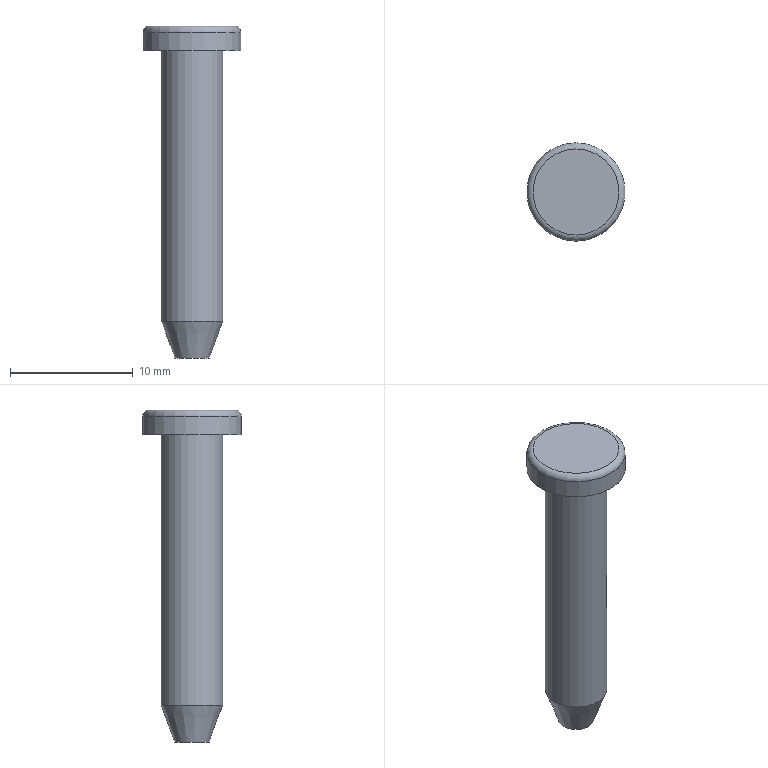Part | STEP file | 1-28.9 | 1 solid | 7 faces | box 8 x 8 x 27 mm | volume 568.112 mm3 | plane 3 | cylinder 2 | torus 1 | cone 1 | commonest cylinder face diameters 5 x1 8 x1
STEP:
#1=CARTESIAN_POINT('',(0.,0.,0.));
#2=DIRECTION('',(0.,0.,1.));
#3=DIRECTION('',(1.,0.,0.));
#4=AXIS2_PLACEMENT_3D('',#1,#2,#3);
#5=CARTESIAN_POINT('',(0.,4.,0.));
#6=VERTEX_POINT('',#5);
#7=CARTESIAN_POINT('',(0.,0.,0.));
#8=DIRECTION('',(0.,0.,1.));
#9=DIRECTION('',(0.,1.,0.));
#10=AXIS2_PLACEMENT_3D('',#7,#8,#9);
#11=CIRCLE('',#10,4.);
#12=CARTESIAN_POINT('',(0.,-1.072,0.));
#13=DIRECTION('',(0.,0.,1.));
#14=DIRECTION('',(1.,0.,0.));
#15=AXIS2_PLACEMENT_3D('',#12,#13,#14);
#16=PLANE('',#15);
#17=CARTESIAN_POINT('',(0.,1.072));
#18=DIRECTION('',(0.,1.));
#19=AXIS2_PLACEMENT_2D('',#17,#18);
#20=CIRCLE('',#19,4.);
#21=(GEOMETRIC_REPRESENTATION_CONTEXT(2)PARAMETRIC_REPRESENTATION_CONTEXT()REPRESENTATION_CONTEXT('',''));
#22=DEFINITIONAL_REPRESENTATION('',(#20),#21);
#23=PCURVE('',#16,#22);
#24=CARTESIAN_POINT('',(0.,0.,0.));
#25=DIRECTION('',(0.,0.,1.));
#26=DIRECTION('',(0.,1.,0.));
#27=AXIS2_PLACEMENT_3D('',#24,#25,#26);
#28=CYLINDRICAL_SURFACE('',#27,4.);
#29=CARTESIAN_POINT('',(0.,0.));
#30=DIRECTION('',(1.,0.));
#31=VECTOR('',#30,1.);
#32=LINE('',#29,#31);
#33=(GEOMETRIC_REPRESENTATION_CONTEXT(2)PARAMETRIC_REPRESENTATION_CONTEXT()REPRESENTATION_CONTEXT('',''));
#34=DEFINITIONAL_REPRESENTATION('',(#32),#33);
#35=PCURVE('',#28,#34);
#36=SURFACE_CURVE('',#11,(#23,#35),.PCURVE_S1.);
#37=EDGE_CURVE('',#6,#6,#36,.T.);
#38=ORIENTED_EDGE('',*,*,#37,.T.);
#39=EDGE_LOOP('',(#38));
#40=FACE_BOUND('',#39,.F.);
#41=CARTESIAN_POINT('',(0.,2.5,0.));
#42=VERTEX_POINT('',#41);
#43=CARTESIAN_POINT('',(0.,0.,0.));
#44=DIRECTION('',(0.,0.,1.));
#45=DIRECTION('',(0.,1.,0.));
#46=AXIS2_PLACEMENT_3D('',#43,#44,#45);
#47=CIRCLE('',#46,2.5);
#48=CARTESIAN_POINT('',(0.,1.072));
#49=DIRECTION('',(0.,1.));
#50=AXIS2_PLACEMENT_2D('',#48,#49);
#51=CIRCLE('',#50,2.5);
#52=(GEOMETRIC_REPRESENTATION_CONTEXT(2)PARAMETRIC_REPRESENTATION_CONTEXT()REPRESENTATION_CONTEXT('',''));
#53=DEFINITIONAL_REPRESENTATION('',(#51),#52);
#54=PCURVE('',#16,#53);
#55=CARTESIAN_POINT('',(0.,0.,0.));
#56=DIRECTION('',(0.,0.,-1.));
#57=DIRECTION('',(0.,1.,0.));
#58=AXIS2_PLACEMENT_3D('',#55,#56,#57);
#59=CYLINDRICAL_SURFACE('',#58,2.5);
#60=CARTESIAN_POINT('',(6.283,0.));
#61=DIRECTION('',(-1.,0.));
#62=VECTOR('',#61,1.);
#63=LINE('',#60,#62);
#64=(GEOMETRIC_REPRESENTATION_CONTEXT(2)PARAMETRIC_REPRESENTATION_CONTEXT()REPRESENTATION_CONTEXT('',''));
#65=DEFINITIONAL_REPRESENTATION('',(#63),#64);
#66=PCURVE('',#59,#65);
#67=SURFACE_CURVE('',#47,(#54,#66),.PCURVE_S1.);
#68=EDGE_CURVE('',#42,#42,#67,.T.);
#69=ORIENTED_EDGE('',*,*,#68,.F.);
#70=EDGE_LOOP('',(#69));
#71=FACE_BOUND('',#70,.F.);
#72=ADVANCED_FACE('',(#40,#71),#16,.F.);
#73=CARTESIAN_POINT('',(0.,2.5,-22.));
#74=VERTEX_POINT('',#73);
#75=CARTESIAN_POINT('',(0.,2.5,0.));
#76=DIRECTION('',(0.,0.,-1.));
#77=VECTOR('',#76,1.);
#78=LINE('',#75,#77);
#79=CARTESIAN_POINT('',(6.283,0.));
#80=DIRECTION('',(0.,1.));
#81=VECTOR('',#80,1.);
#82=LINE('',#79,#81);
#83=(GEOMETRIC_REPRESENTATION_CONTEXT(2)PARAMETRIC_REPRESENTATION_CONTEXT()REPRESENTATION_CONTEXT('',''));
#84=DEFINITIONAL_REPRESENTATION('',(#82),#83);
#85=PCURVE('',#59,#84);
#86=CARTESIAN_POINT('',(0.,0.));
#87=DIRECTION('',(0.,1.));
#88=VECTOR('',#87,1.);
#89=LINE('',#86,#88);
#90=(GEOMETRIC_REPRESENTATION_CONTEXT(2)PARAMETRIC_REPRESENTATION_CONTEXT()REPRESENTATION_CONTEXT('',''));
#91=DEFINITIONAL_REPRESENTATION('',(#89),#90);
#92=PCURVE('',#59,#91);
#93=SEAM_CURVE('',#78,(#85,#92),.PCURVE_S1.);
#94=EDGE_CURVE('',#42,#74,#93,.T.);
#95=ORIENTED_EDGE('',*,*,#94,.T.);
#96=CARTESIAN_POINT('',(0.,0.,-22.));
#97=DIRECTION('',(0.,0.,1.));
#98=DIRECTION('',(0.,1.,0.));
#99=AXIS2_PLACEMENT_3D('',#96,#97,#98);
#100=CIRCLE('',#99,2.5);
#101=CARTESIAN_POINT('',(6.283,22.));
#102=DIRECTION('',(-1.,0.));
#103=VECTOR('',#102,1.);
#104=LINE('',#101,#103);
#105=(GEOMETRIC_REPRESENTATION_CONTEXT(2)PARAMETRIC_REPRESENTATION_CONTEXT()REPRESENTATION_CONTEXT('',''));
#106=DEFINITIONAL_REPRESENTATION('',(#104),#105);
#107=PCURVE('',#59,#106);
#108=CARTESIAN_POINT('',(0.,0.,-25.));
#109=DIRECTION('',(0.,0.,1.));
#110=DIRECTION('',(0.,1.,0.));
#111=AXIS2_PLACEMENT_3D('',#108,#109,#110);
#112=CONICAL_SURFACE('',#111,1.408,0.3491);
#113=CARTESIAN_POINT('',(0.,3.));
#114=DIRECTION('',(1.,0.));
#115=VECTOR('',#114,1.);
#116=LINE('',#113,#115);
#117=(GEOMETRIC_REPRESENTATION_CONTEXT(2)PARAMETRIC_REPRESENTATION_CONTEXT()REPRESENTATION_CONTEXT('',''));
#118=DEFINITIONAL_REPRESENTATION('',(#116),#117);
#119=PCURVE('',#112,#118);
#120=SURFACE_CURVE('',#100,(#107,#119),.PCURVE_S1.);
#121=EDGE_CURVE('',#74,#74,#120,.T.);
#122=ORIENTED_EDGE('',*,*,#121,.T.);
#123=ORIENTED_EDGE('',*,*,#94,.F.);
#124=ORIENTED_EDGE('',*,*,#68,.F.);
#125=EDGE_LOOP('',(#95,#122,#123,#124));
#126=FACE_BOUND('',#125,.T.);
#127=ADVANCED_FACE('',(#126),#59,.T.);
#128=CARTESIAN_POINT('',(0.,3.5,2.));
#129=VERTEX_POINT('',#128);
#130=CARTESIAN_POINT('',(0.,0.,2.));
#131=DIRECTION('',(0.,0.,-1.));
#132=DIRECTION('',(0.,1.,0.));
#133=AXIS2_PLACEMENT_3D('',#130,#131,#132);
#134=CIRCLE('',#133,3.5);
#135=CARTESIAN_POINT('',(0.,-1.072,2.));
#136=DIRECTION('',(0.,0.,1.));
#137=DIRECTION('',(1.,0.,0.));
#138=AXIS2_PLACEMENT_3D('',#135,#136,#137);
#139=PLANE('',#138);
#140=CARTESIAN_POINT('',(0.,4.572));
#141=CARTESIAN_POINT('',(6.062,4.572));
#142=CARTESIAN_POINT('',(3.031,-0.6782));
#143=CARTESIAN_POINT('',(0.,-5.928));
#144=CARTESIAN_POINT('',(-3.031,-0.6782));
#145=CARTESIAN_POINT('',(-6.062,4.572));
#146=CARTESIAN_POINT('',(0.,4.572));
#147=(BOUNDED_CURVE()B_SPLINE_CURVE(2,(#140,#141,#142,#143,#144,#145,#146),.UNSPECIFIED.,.T.,.F.)B_SPLINE_CURVE_WITH_KNOTS((1,2,2,2,2,1),(-2.094,0.,2.094,4.189,6.283,8.378),.UNSPECIFIED.)CURVE()GEOMETRIC_REPRESENTATION_ITEM()RATIONAL_B_SPLINE_CURVE((1.,0.5,1.,0.5,1.,0.5,1.))REPRESENTATION_ITEM(''));
#148=(GEOMETRIC_REPRESENTATION_CONTEXT(2)PARAMETRIC_REPRESENTATION_CONTEXT()REPRESENTATION_CONTEXT('',''));
#149=DEFINITIONAL_REPRESENTATION('',(#147),#148);
#150=PCURVE('',#139,#149);
#151=CARTESIAN_POINT('',(0.,0.,1.5));
#152=DIRECTION('',(0.,0.,1.));
#153=DIRECTION('',(0.,1.,0.));
#154=AXIS2_PLACEMENT_3D('',#151,#152,#153);
#155=TOROIDAL_SURFACE('',#154,3.5,0.5);
#156=CARTESIAN_POINT('',(6.283,1.571));
#157=DIRECTION('',(-1.,0.));
#158=VECTOR('',#157,1.);
#159=LINE('',#156,#158);
#160=(GEOMETRIC_REPRESENTATION_CONTEXT(2)PARAMETRIC_REPRESENTATION_CONTEXT()REPRESENTATION_CONTEXT('',''));
#161=DEFINITIONAL_REPRESENTATION('',(#159),#160);
#162=PCURVE('',#155,#161);
#163=SURFACE_CURVE('',#134,(#150,#162),.PCURVE_S1.);
#164=EDGE_CURVE('',#129,#129,#163,.T.);
#165=ORIENTED_EDGE('',*,*,#164,.F.);
#166=EDGE_LOOP('',(#165));
#167=FACE_BOUND('',#166,.T.);
#168=ADVANCED_FACE('',(#167),#139,.T.);
#169=ORIENTED_EDGE('',*,*,#37,.T.);
#170=CARTESIAN_POINT('',(0.,4.,1.5));
#171=VERTEX_POINT('',#170);
#172=CARTESIAN_POINT('',(0.,4.,0.));
#173=DIRECTION('',(0.,0.,1.));
#174=VECTOR('',#173,1.);
#175=LINE('',#172,#174);
#176=CARTESIAN_POINT('',(6.283,0.));
#177=DIRECTION('',(0.,1.));
#178=VECTOR('',#177,1.);
#179=LINE('',#176,#178);
#180=(GEOMETRIC_REPRESENTATION_CONTEXT(2)PARAMETRIC_REPRESENTATION_CONTEXT()REPRESENTATION_CONTEXT('',''));
#181=DEFINITIONAL_REPRESENTATION('',(#179),#180);
#182=PCURVE('',#28,#181);
#183=CARTESIAN_POINT('',(0.,0.));
#184=DIRECTION('',(0.,1.));
#185=VECTOR('',#184,1.);
#186=LINE('',#183,#185);
#187=(GEOMETRIC_REPRESENTATION_CONTEXT(2)PARAMETRIC_REPRESENTATION_CONTEXT()REPRESENTATION_CONTEXT('',''));
#188=DEFINITIONAL_REPRESENTATION('',(#186),#187);
#189=PCURVE('',#28,#188);
#190=SEAM_CURVE('',#175,(#182,#189),.PCURVE_S1.);
#191=EDGE_CURVE('',#6,#171,#190,.T.);
#192=ORIENTED_EDGE('',*,*,#191,.T.);
#193=CARTESIAN_POINT('',(0.,0.,1.5));
#194=DIRECTION('',(0.,0.,-1.));
#195=DIRECTION('',(0.,1.,0.));
#196=AXIS2_PLACEMENT_3D('',#193,#194,#195);
#197=CIRCLE('',#196,4.);
#198=CARTESIAN_POINT('',(6.283,1.5));
#199=DIRECTION('',(-1.,0.));
#200=VECTOR('',#199,1.);
#201=LINE('',#198,#200);
#202=(GEOMETRIC_REPRESENTATION_CONTEXT(2)PARAMETRIC_REPRESENTATION_CONTEXT()REPRESENTATION_CONTEXT('',''));
#203=DEFINITIONAL_REPRESENTATION('',(#201),#202);
#204=PCURVE('',#28,#203);
#205=CARTESIAN_POINT('',(6.283,0.));
#206=DIRECTION('',(-1.,0.));
#207=VECTOR('',#206,1.);
#208=LINE('',#205,#207);
#209=(GEOMETRIC_REPRESENTATION_CONTEXT(2)PARAMETRIC_REPRESENTATION_CONTEXT()REPRESENTATION_CONTEXT('',''));
#210=DEFINITIONAL_REPRESENTATION('',(#208),#209);
#211=PCURVE('',#155,#210);
#212=SURFACE_CURVE('',#197,(#204,#211),.PCURVE_S1.);
#213=EDGE_CURVE('',#171,#171,#212,.T.);
#214=ORIENTED_EDGE('',*,*,#213,.T.);
#215=ORIENTED_EDGE('',*,*,#191,.F.);
#216=EDGE_LOOP('',(#169,#192,#214,#215));
#217=FACE_BOUND('',#216,.T.);
#218=ADVANCED_FACE('',(#217),#28,.T.);
#219=CARTESIAN_POINT('',(0.,3.5,1.5));
#220=DIRECTION('',(-1.,0.,0.));
#221=DIRECTION('',(0.,0.,1.));
#222=AXIS2_PLACEMENT_3D('',#219,#220,#221);
#223=CIRCLE('',#222,0.5);
#224=CARTESIAN_POINT('',(0.,1.571));
#225=DIRECTION('',(0.,-1.));
#226=VECTOR('',#225,1.);
#227=LINE('',#224,#226);
#228=(GEOMETRIC_REPRESENTATION_CONTEXT(2)PARAMETRIC_REPRESENTATION_CONTEXT()REPRESENTATION_CONTEXT('',''));
#229=DEFINITIONAL_REPRESENTATION('',(#227),#228);
#230=PCURVE('',#155,#229);
#231=CARTESIAN_POINT('',(6.283,1.571));
#232=DIRECTION('',(0.,-1.));
#233=VECTOR('',#232,1.);
#234=LINE('',#231,#233);
#235=(GEOMETRIC_REPRESENTATION_CONTEXT(2)PARAMETRIC_REPRESENTATION_CONTEXT()REPRESENTATION_CONTEXT('',''));
#236=DEFINITIONAL_REPRESENTATION('',(#234),#235);
#237=PCURVE('',#155,#236);
#238=SEAM_CURVE('',#223,(#230,#237),.PCURVE_S1.);
#239=EDGE_CURVE('',#129,#171,#238,.T.);
#240=ORIENTED_EDGE('',*,*,#239,.T.);
#241=ORIENTED_EDGE('',*,*,#213,.F.);
#242=ORIENTED_EDGE('',*,*,#239,.F.);
#243=ORIENTED_EDGE('',*,*,#164,.T.);
#244=EDGE_LOOP('',(#240,#241,#242,#243));
#245=FACE_BOUND('',#244,.T.);
#246=ADVANCED_FACE('',(#245),#155,.T.);
#247=CARTESIAN_POINT('',(0.,1.408,-25.));
#248=VERTEX_POINT('',#247);
#249=CARTESIAN_POINT('',(0.,0.,-25.));
#250=DIRECTION('',(0.,0.,1.));
#251=DIRECTION('',(0.,1.,0.));
#252=AXIS2_PLACEMENT_3D('',#249,#250,#251);
#253=CIRCLE('',#252,1.408);
#254=CARTESIAN_POINT('',(0.,0.));
#255=DIRECTION('',(1.,0.));
#256=VECTOR('',#255,1.);
#257=LINE('',#254,#256);
#258=(GEOMETRIC_REPRESENTATION_CONTEXT(2)PARAMETRIC_REPRESENTATION_CONTEXT()REPRESENTATION_CONTEXT('',''));
#259=DEFINITIONAL_REPRESENTATION('',(#257),#258);
#260=PCURVE('',#112,#259);
#261=CARTESIAN_POINT('',(0.,0.,-25.));
#262=DIRECTION('',(0.,0.,1.));
#263=DIRECTION('',(0.,1.,0.));
#264=AXIS2_PLACEMENT_3D('',#261,#262,#263);
#265=PLANE('',#264);
#266=CARTESIAN_POINT('',(0.,0.));
#267=DIRECTION('',(1.,0.));
#268=AXIS2_PLACEMENT_2D('',#266,#267);
#269=CIRCLE('',#268,1.408);
#270=(GEOMETRIC_REPRESENTATION_CONTEXT(2)PARAMETRIC_REPRESENTATION_CONTEXT()REPRESENTATION_CONTEXT('',''));
#271=DEFINITIONAL_REPRESENTATION('',(#269),#270);
#272=PCURVE('',#265,#271);
#273=SURFACE_CURVE('',#253,(#260,#272),.PCURVE_S1.);
#274=EDGE_CURVE('',#248,#248,#273,.T.);
#275=ORIENTED_EDGE('',*,*,#274,.T.);
#276=CARTESIAN_POINT('',(0.,1.408,-25.));
#277=DIRECTION('',(0.,0.342,0.9397));
#278=VECTOR('',#277,1.);
#279=LINE('',#276,#278);
#280=CARTESIAN_POINT('',(6.283,0.));
#281=DIRECTION('',(0.,1.));
#282=VECTOR('',#281,1.);
#283=LINE('',#280,#282);
#284=(GEOMETRIC_REPRESENTATION_CONTEXT(2)PARAMETRIC_REPRESENTATION_CONTEXT()REPRESENTATION_CONTEXT('',''));
#285=DEFINITIONAL_REPRESENTATION('',(#283),#284);
#286=PCURVE('',#112,#285);
#287=CARTESIAN_POINT('',(0.,0.));
#288=DIRECTION('',(0.,1.));
#289=VECTOR('',#288,1.);
#290=LINE('',#287,#289);
#291=(GEOMETRIC_REPRESENTATION_CONTEXT(2)PARAMETRIC_REPRESENTATION_CONTEXT()REPRESENTATION_CONTEXT('',''));
#292=DEFINITIONAL_REPRESENTATION('',(#290),#291);
#293=PCURVE('',#112,#292);
#294=SEAM_CURVE('',#279,(#286,#293),.PCURVE_S1.);
#295=EDGE_CURVE('',#248,#74,#294,.T.);
#296=ORIENTED_EDGE('',*,*,#295,.T.);
#297=ORIENTED_EDGE('',*,*,#121,.F.);
#298=ORIENTED_EDGE('',*,*,#295,.F.);
#299=EDGE_LOOP('',(#275,#296,#297,#298));
#300=FACE_BOUND('',#299,.T.);
#301=ADVANCED_FACE('',(#300),#112,.T.);
#302=ORIENTED_EDGE('',*,*,#274,.T.);
#303=EDGE_LOOP('',(#302));
#304=FACE_BOUND('',#303,.F.);
#305=ADVANCED_FACE('',(#304),#265,.F.);
#306=CLOSED_SHELL('',(#72,#127,#168,#218,#246,#301,#305));
#307=MANIFOLD_SOLID_BREP('',#306);
#308=(LENGTH_UNIT()NAMED_UNIT(*)SI_UNIT(.MILLI.,.METRE.));
#309=UNCERTAINTY_MEASURE_WITH_UNIT(LENGTH_MEASURE(0.0000001),#308,'','');
#310=(NAMED_UNIT(*)PLANE_ANGLE_UNIT()SI_UNIT($,.RADIAN.));
#311=(NAMED_UNIT(*)SI_UNIT($,.STERADIAN.)SOLID_ANGLE_UNIT());
#312=(GEOMETRIC_REPRESENTATION_CONTEXT(3)GLOBAL_UNCERTAINTY_ASSIGNED_CONTEXT((#309))GLOBAL_UNIT_ASSIGNED_CONTEXT((#308,#310,#311))REPRESENTATION_CONTEXT('',''));
#313=ADVANCED_BREP_SHAPE_REPRESENTATION('',(#4,#307),#312);